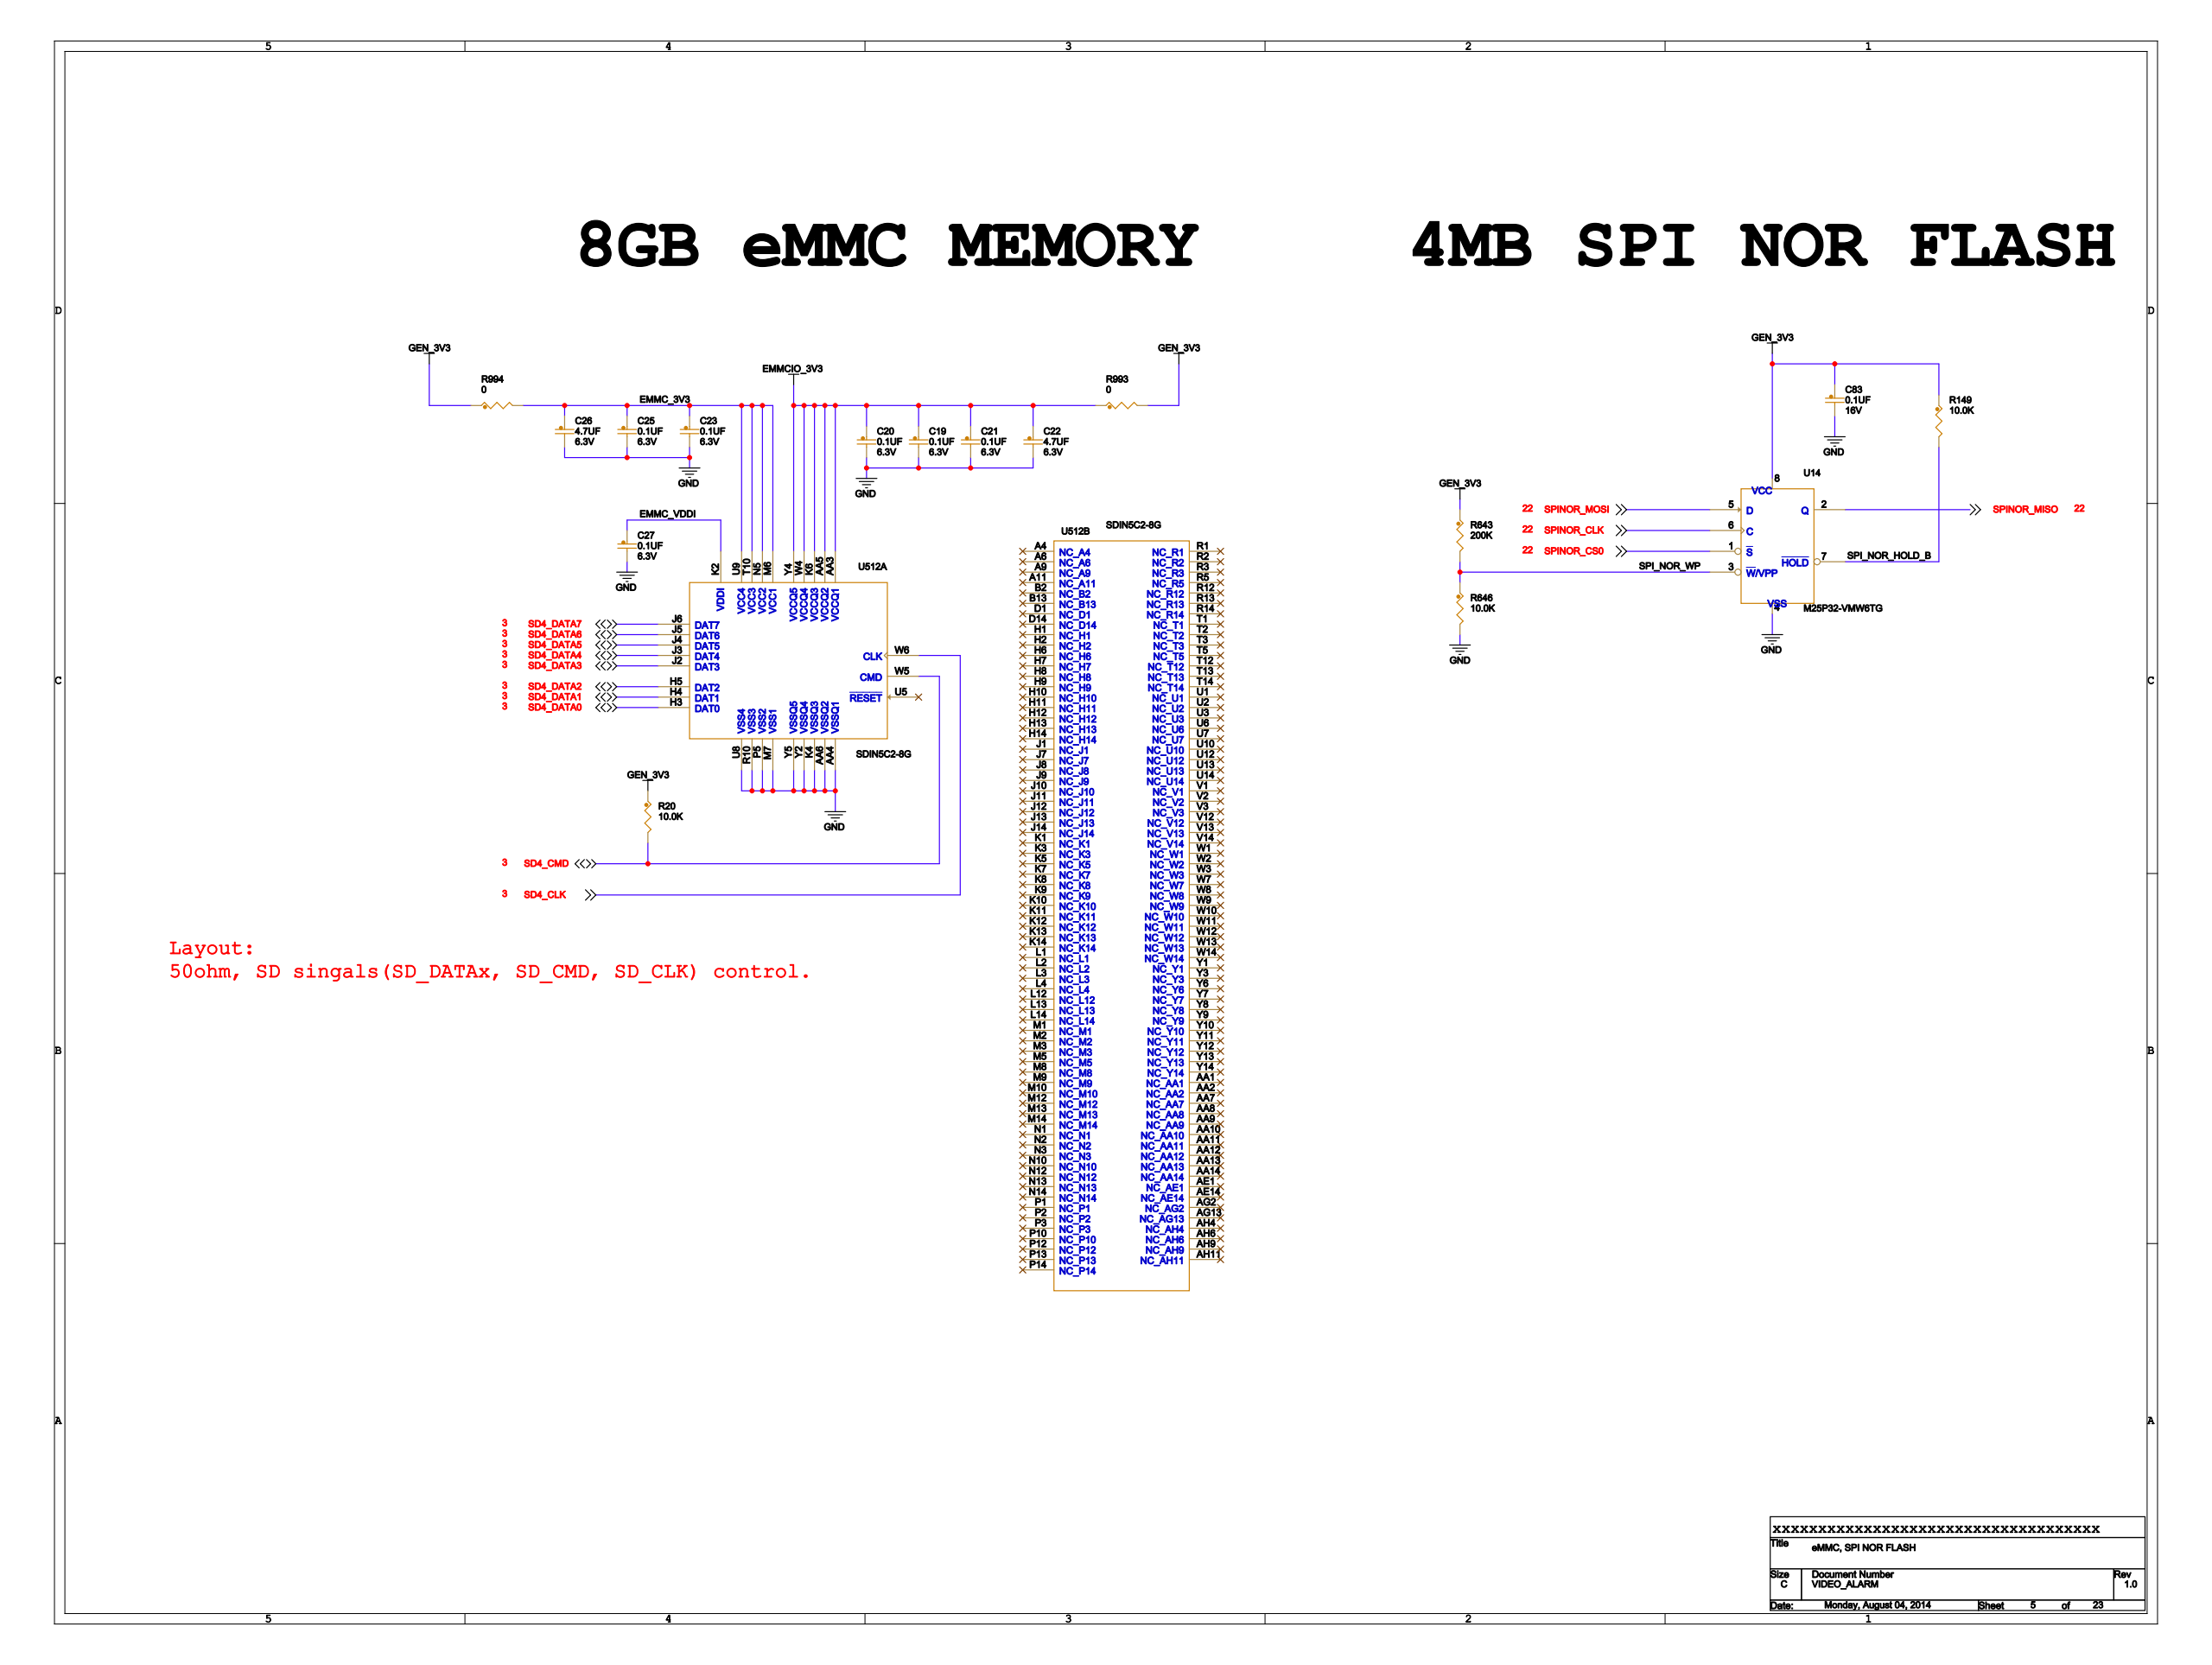Circuit board | Cadence Allegro | 994 parts | 728 nets | one sheet of the schematic
Parts on this sheet (reference | value | footprint):
C19 | 0.1UF | 0603_CC
C20 | 0.1UF | 0603_CC
C21 | 0.1UF | 0603_CC
C22 | 4.7UF | 0603_CC
C23 | 0.1UF | 0603_CC
C25 | 0.1UF | 0603_CC
C26 | 4.7UF | 0603_CC
C27 | 0.1UF | 0603_CC
C83 | 0.1UF | 0603_CC
J8 | 10029449-001RLF | HDMI
R20 | 10.0K | 0603_CC
R149 | 10.0K | 0603_CC
R643 | 200K | 0603_CC
R646 | 10.0K | 0603_CC
R993 | 0 | 0603_CC
R994 | 0 | 0603_CC
U1 | MCIMX6Q6AVT10AC | BGA624_0P8_21X21
U2 | MT41K128M16JT | BGA96_0P8_8P15X14P15
U3 | MT41K128M16JT | BGA96_0P8_8P15X14P15
U5 | MT41K128M16JT | BGA96_0P8_8P15X14P15
U8 | MMPF0100F0EP | QFN56_0P5_8X8_EP4P5
U14 | M25P32-VMW6TG | SO8WST
U512 | SDIN5C2-8G | BGA169_0P5_12X16
Nets of these parts (net: part-pin ...):
GND: C19-2 C20-2 C21-2 C22-2 C23-2 C25-2 C26-2 C27-2 C83-2 R646-2 U14-4 J8-2 J8-5 J8-8 U1-A4 U1-AA7 U1-AA10 U1-AA13 U1-AE1 U1-H8 U1-H12 U1-J2 U1-J8 U1-J12 U1-K8 U1-K10 U1-K12 U1-L2 U1-L12 U1-M8 U1-M10 U1-M12 U1-N10 U1-P10 U1-P12 U1-R12 U1-T12 U1-U8 U1-U12 U1-W3 U1-W7 U1-W8 U1-W9 U1-W10 U1-W11 U1-W12 U1-W13 U1-Y5 U2-A9 U2-D1 U2-J2 U2-J8 U2-M1 U2-M9 U2-P1 U2-T1 U3-A9 U3-D1 U3-J2 U3-J8 U3-M1 U3-M9 U3-P1 U3-T1 U5-A9 U5-D1 U5-J2 U5-J8 U5-M1 U5-M9 U5-P1 U5-T1 U8-5 U512-AA4 U512-AA6 U512-K4 U512-M7 U512-P5 U512-R10 U512-U8 U512-Y2 U512-Y5
GEN_3V3: C83-1 R20-1 R149-1 R643-1 R993-2 R994-1 U14-8
EMMC_3V3: C23-1 C25-1 C26-1 R994-2 U512-M6 U512-N5 U512-T10 U512-U9
EMMCIO_3V3: C19-1 C20-1 C21-1 C22-1 R993-1 U512-AA3 U512-AA5 U512-K6 U512-W4 U512-Y4
SPI_NOR_WP: R643-2 R646-1 U14-3
SD4_CMD: R20-2 U512-W5
SPI_NOR_HOLD_B: R149-2 U14-7
EMMC_VDDI: C27-1 U512-K2
SD4_CLK: U512-W6
SD4_DATA0: U512-H3
SD4_DATA1: U512-H4
SD4_DATA2: U512-H5
SD4_DATA3: U512-J2
SD4_DATA4: U512-J3
SD4_DATA5: U1-C19 U512-J4
SD4_DATA6: U512-J5
SD4_DATA7: U512-J6
SPINOR_CLK: U14-6
SPINOR_MOSI: U14-5
SPINOR_MISO: U14-2
SPINOR_CS0: U14-1